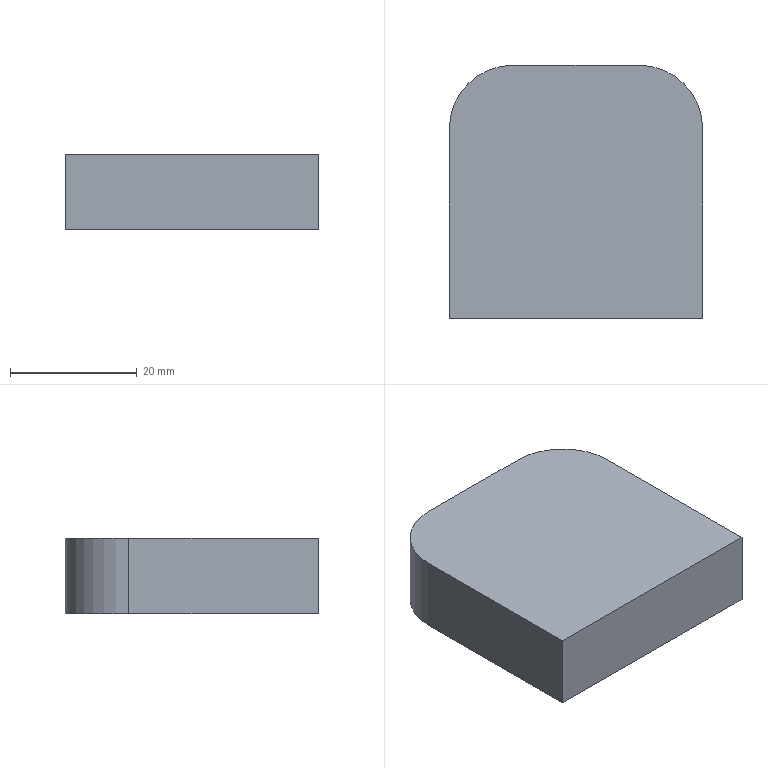Part | SolidWorks | features Extrusion 1 | 1 solid | 8 faces | box 40 x 40 x 12 mm | volume 18685 mm3 | plane 6 | cylinder 2 | commonest cylinder face diameters 20 x2
STEP:
#1=CARTESIAN_POINT('',(0.,30.,0.));
#2=VERTEX_POINT('',#1);
#3=CARTESIAN_POINT('',(0.,0.,0.));
#4=VERTEX_POINT('',#3);
#5=CARTESIAN_POINT('',(0.,0.,0.));
#6=DIRECTION('',(0.,-1.,0.));
#7=VECTOR('',#6,1000.);
#8=LINE('',#5,#7);
#9=EDGE_CURVE('',#2,#4,#8,.T.);
#10=ORIENTED_EDGE('',*,*,#9,.T.);
#11=CARTESIAN_POINT('',(0.,0.,12.));
#12=VERTEX_POINT('',#11);
#13=CARTESIAN_POINT('',(0.,0.,12.));
#14=DIRECTION('',(0.,0.,-1.));
#15=VECTOR('',#14,1000.);
#16=LINE('',#13,#15);
#17=EDGE_CURVE('',#12,#4,#16,.T.);
#18=ORIENTED_EDGE('',*,*,#17,.F.);
#19=CARTESIAN_POINT('',(0.,30.,12.));
#20=VERTEX_POINT('',#19);
#21=CARTESIAN_POINT('',(0.,0.,12.));
#22=DIRECTION('',(0.,-1.,0.));
#23=VECTOR('',#22,1000.);
#24=LINE('',#21,#23);
#25=EDGE_CURVE('',#20,#12,#24,.T.);
#26=ORIENTED_EDGE('',*,*,#25,.F.);
#27=CARTESIAN_POINT('',(0.,30.,12.));
#28=DIRECTION('',(0.,0.,-1.));
#29=VECTOR('',#28,1000.);
#30=LINE('',#27,#29);
#31=EDGE_CURVE('',#20,#2,#30,.T.);
#32=ORIENTED_EDGE('',*,*,#31,.T.);
#33=EDGE_LOOP('',(#10,#18,#26,#32));
#34=FACE_OUTER_BOUND('',#33,.T.);
#35=CARTESIAN_POINT('',(0.,0.,12.));
#36=DIRECTION('',(1.,0.,0.));
#37=DIRECTION('',(0.,0.,-1.));
#38=AXIS2_PLACEMENT_3D('',#35,#36,#37);
#39=PLANE('',#38);
#40=ADVANCED_FACE('',(#34),#39,.F.);
#41=CARTESIAN_POINT('',(40.,0.,0.));
#42=VERTEX_POINT('',#41);
#43=CARTESIAN_POINT('',(0.,0.,0.));
#44=DIRECTION('',(1.,0.,0.));
#45=VECTOR('',#44,1000.);
#46=LINE('',#43,#45);
#47=EDGE_CURVE('',#4,#42,#46,.T.);
#48=ORIENTED_EDGE('',*,*,#47,.T.);
#49=CARTESIAN_POINT('',(40.,0.,12.));
#50=VERTEX_POINT('',#49);
#51=CARTESIAN_POINT('',(40.,0.,12.));
#52=DIRECTION('',(0.,0.,-1.));
#53=VECTOR('',#52,1000.);
#54=LINE('',#51,#53);
#55=EDGE_CURVE('',#50,#42,#54,.T.);
#56=ORIENTED_EDGE('',*,*,#55,.F.);
#57=CARTESIAN_POINT('',(0.,0.,12.));
#58=DIRECTION('',(1.,0.,0.));
#59=VECTOR('',#58,1000.);
#60=LINE('',#57,#59);
#61=EDGE_CURVE('',#12,#50,#60,.T.);
#62=ORIENTED_EDGE('',*,*,#61,.F.);
#63=ORIENTED_EDGE('',*,*,#17,.T.);
#64=EDGE_LOOP('',(#48,#56,#62,#63));
#65=FACE_OUTER_BOUND('',#64,.T.);
#66=CARTESIAN_POINT('',(0.,0.,12.));
#67=DIRECTION('',(0.,1.,0.));
#68=DIRECTION('',(0.,0.,1.));
#69=AXIS2_PLACEMENT_3D('',#66,#67,#68);
#70=PLANE('',#69);
#71=ADVANCED_FACE('',(#65),#70,.F.);
#72=CARTESIAN_POINT('',(40.,30.,0.));
#73=VERTEX_POINT('',#72);
#74=CARTESIAN_POINT('',(40.,0.,0.));
#75=DIRECTION('',(0.,1.,0.));
#76=VECTOR('',#75,1000.);
#77=LINE('',#74,#76);
#78=EDGE_CURVE('',#42,#73,#77,.T.);
#79=ORIENTED_EDGE('',*,*,#78,.T.);
#80=CARTESIAN_POINT('',(40.,30.,12.));
#81=VERTEX_POINT('',#80);
#82=CARTESIAN_POINT('',(40.,30.,12.));
#83=DIRECTION('',(0.,0.,-1.));
#84=VECTOR('',#83,1000.);
#85=LINE('',#82,#84);
#86=EDGE_CURVE('',#81,#73,#85,.T.);
#87=ORIENTED_EDGE('',*,*,#86,.F.);
#88=CARTESIAN_POINT('',(40.,0.,12.));
#89=DIRECTION('',(0.,1.,0.));
#90=VECTOR('',#89,1000.);
#91=LINE('',#88,#90);
#92=EDGE_CURVE('',#50,#81,#91,.T.);
#93=ORIENTED_EDGE('',*,*,#92,.F.);
#94=ORIENTED_EDGE('',*,*,#55,.T.);
#95=EDGE_LOOP('',(#79,#87,#93,#94));
#96=FACE_OUTER_BOUND('',#95,.T.);
#97=CARTESIAN_POINT('',(40.,0.,12.));
#98=DIRECTION('',(-1.,0.,0.));
#99=DIRECTION('',(0.,0.,1.));
#100=AXIS2_PLACEMENT_3D('',#97,#98,#99);
#101=PLANE('',#100);
#102=ADVANCED_FACE('',(#96),#101,.F.);
#103=CARTESIAN_POINT('',(30.,40.,0.));
#104=VERTEX_POINT('',#103);
#105=CARTESIAN_POINT('',(30.,30.,0.));
#106=DIRECTION('',(0.,0.,1.));
#107=DIRECTION('',(1.,0.,0.));
#108=AXIS2_PLACEMENT_3D('',#105,#106,#107);
#109=CIRCLE('',#108,10.);
#110=EDGE_CURVE('',#73,#104,#109,.T.);
#111=ORIENTED_EDGE('',*,*,#110,.T.);
#112=CARTESIAN_POINT('',(30.,40.,12.));
#113=VERTEX_POINT('',#112);
#114=CARTESIAN_POINT('',(30.,40.,12.));
#115=DIRECTION('',(0.,0.,-1.));
#116=VECTOR('',#115,1000.);
#117=LINE('',#114,#116);
#118=EDGE_CURVE('',#113,#104,#117,.T.);
#119=ORIENTED_EDGE('',*,*,#118,.F.);
#120=CARTESIAN_POINT('',(30.,30.,12.));
#121=DIRECTION('',(0.,0.,1.));
#122=DIRECTION('',(1.,0.,0.));
#123=AXIS2_PLACEMENT_3D('',#120,#121,#122);
#124=CIRCLE('',#123,10.);
#125=EDGE_CURVE('',#81,#113,#124,.T.);
#126=ORIENTED_EDGE('',*,*,#125,.F.);
#127=ORIENTED_EDGE('',*,*,#86,.T.);
#128=EDGE_LOOP('',(#111,#119,#126,#127));
#129=FACE_OUTER_BOUND('',#128,.T.);
#130=CARTESIAN_POINT('',(30.,30.,12.));
#131=DIRECTION('',(0.,0.,-1.));
#132=DIRECTION('',(-1.,0.,0.));
#133=AXIS2_PLACEMENT_3D('',#130,#131,#132);
#134=CYLINDRICAL_SURFACE('',#133,10.);
#135=ADVANCED_FACE('',(#129),#134,.T.);
#136=CARTESIAN_POINT('',(10.,40.,0.));
#137=VERTEX_POINT('',#136);
#138=CARTESIAN_POINT('',(10.,40.,0.));
#139=DIRECTION('',(-1.,0.,0.));
#140=VECTOR('',#139,1000.);
#141=LINE('',#138,#140);
#142=EDGE_CURVE('',#104,#137,#141,.T.);
#143=ORIENTED_EDGE('',*,*,#142,.T.);
#144=CARTESIAN_POINT('',(10.,40.,12.));
#145=VERTEX_POINT('',#144);
#146=CARTESIAN_POINT('',(10.,40.,12.));
#147=DIRECTION('',(0.,0.,-1.));
#148=VECTOR('',#147,1000.);
#149=LINE('',#146,#148);
#150=EDGE_CURVE('',#145,#137,#149,.T.);
#151=ORIENTED_EDGE('',*,*,#150,.F.);
#152=CARTESIAN_POINT('',(10.,40.,12.));
#153=DIRECTION('',(-1.,0.,0.));
#154=VECTOR('',#153,1000.);
#155=LINE('',#152,#154);
#156=EDGE_CURVE('',#113,#145,#155,.T.);
#157=ORIENTED_EDGE('',*,*,#156,.F.);
#158=ORIENTED_EDGE('',*,*,#118,.T.);
#159=EDGE_LOOP('',(#143,#151,#157,#158));
#160=FACE_OUTER_BOUND('',#159,.T.);
#161=CARTESIAN_POINT('',(10.,40.,12.));
#162=DIRECTION('',(0.,-1.,0.));
#163=DIRECTION('',(0.,0.,-1.));
#164=AXIS2_PLACEMENT_3D('',#161,#162,#163);
#165=PLANE('',#164);
#166=ADVANCED_FACE('',(#160),#165,.F.);
#167=CARTESIAN_POINT('',(10.,30.,0.));
#168=DIRECTION('',(0.,0.,1.));
#169=DIRECTION('',(-1.,0.,0.));
#170=AXIS2_PLACEMENT_3D('',#167,#168,#169);
#171=CIRCLE('',#170,10.);
#172=EDGE_CURVE('',#137,#2,#171,.T.);
#173=ORIENTED_EDGE('',*,*,#172,.T.);
#174=ORIENTED_EDGE('',*,*,#31,.F.);
#175=CARTESIAN_POINT('',(10.,30.,12.));
#176=DIRECTION('',(0.,0.,1.));
#177=DIRECTION('',(-1.,0.,0.));
#178=AXIS2_PLACEMENT_3D('',#175,#176,#177);
#179=CIRCLE('',#178,10.);
#180=EDGE_CURVE('',#145,#20,#179,.T.);
#181=ORIENTED_EDGE('',*,*,#180,.F.);
#182=ORIENTED_EDGE('',*,*,#150,.T.);
#183=EDGE_LOOP('',(#173,#174,#181,#182));
#184=FACE_OUTER_BOUND('',#183,.T.);
#185=CARTESIAN_POINT('',(10.,30.,12.));
#186=DIRECTION('',(0.,0.,-1.));
#187=DIRECTION('',(-1.,0.,0.));
#188=AXIS2_PLACEMENT_3D('',#185,#186,#187);
#189=CYLINDRICAL_SURFACE('',#188,10.);
#190=ADVANCED_FACE('',(#184),#189,.T.);
#191=ORIENTED_EDGE('',*,*,#25,.T.);
#192=ORIENTED_EDGE('',*,*,#61,.T.);
#193=ORIENTED_EDGE('',*,*,#92,.T.);
#194=ORIENTED_EDGE('',*,*,#125,.T.);
#195=ORIENTED_EDGE('',*,*,#156,.T.);
#196=ORIENTED_EDGE('',*,*,#180,.T.);
#197=EDGE_LOOP('',(#191,#192,#193,#194,#195,#196));
#198=FACE_OUTER_BOUND('',#197,.T.);
#199=CARTESIAN_POINT('',(10.,30.,12.));
#200=DIRECTION('',(0.,0.,-1.));
#201=DIRECTION('',(-1.,0.,0.));
#202=AXIS2_PLACEMENT_3D('',#199,#200,#201);
#203=PLANE('',#202);
#204=ADVANCED_FACE('',(#198),#203,.F.);
#205=ORIENTED_EDGE('',*,*,#9,.F.);
#206=ORIENTED_EDGE('',*,*,#172,.F.);
#207=ORIENTED_EDGE('',*,*,#142,.F.);
#208=ORIENTED_EDGE('',*,*,#110,.F.);
#209=ORIENTED_EDGE('',*,*,#78,.F.);
#210=ORIENTED_EDGE('',*,*,#47,.F.);
#211=EDGE_LOOP('',(#205,#206,#207,#208,#209,#210));
#212=FACE_OUTER_BOUND('',#211,.T.);
#213=CARTESIAN_POINT('',(10.,30.,0.));
#214=DIRECTION('',(0.,0.,-1.));
#215=DIRECTION('',(-1.,0.,0.));
#216=AXIS2_PLACEMENT_3D('',#213,#214,#215);
#217=PLANE('',#216);
#218=ADVANCED_FACE('',(#212),#217,.T.);
#219=CLOSED_SHELL('',(#40,#71,#102,#135,#166,#190,#204,#218));
#220=MANIFOLD_SOLID_BREP('',#219);
#221=CARTESIAN_POINT('',(0.,0.,0.));
#222=DIRECTION('',(0.,0.,1.));
#223=DIRECTION('',(1.,0.,0.));
#224=AXIS2_PLACEMENT_3D('',#221,#222,#223);
#225=(LENGTH_UNIT()NAMED_UNIT(*)SI_UNIT(.MILLI.,.METRE.));
#226=UNCERTAINTY_MEASURE_WITH_UNIT(LENGTH_MEASURE(0.00001),#225,'','');
#227=(NAMED_UNIT(*)PLANE_ANGLE_UNIT()SI_UNIT($,.RADIAN.));
#228=(NAMED_UNIT(*)SI_UNIT($,.STERADIAN.)SOLID_ANGLE_UNIT());
#229=(GEOMETRIC_REPRESENTATION_CONTEXT(3)GLOBAL_UNCERTAINTY_ASSIGNED_CONTEXT((#226))GLOBAL_UNIT_ASSIGNED_CONTEXT((#225,#227,#228))REPRESENTATION_CONTEXT('',''));
#230=ADVANCED_BREP_SHAPE_REPRESENTATION('',(#220,#224),#229);